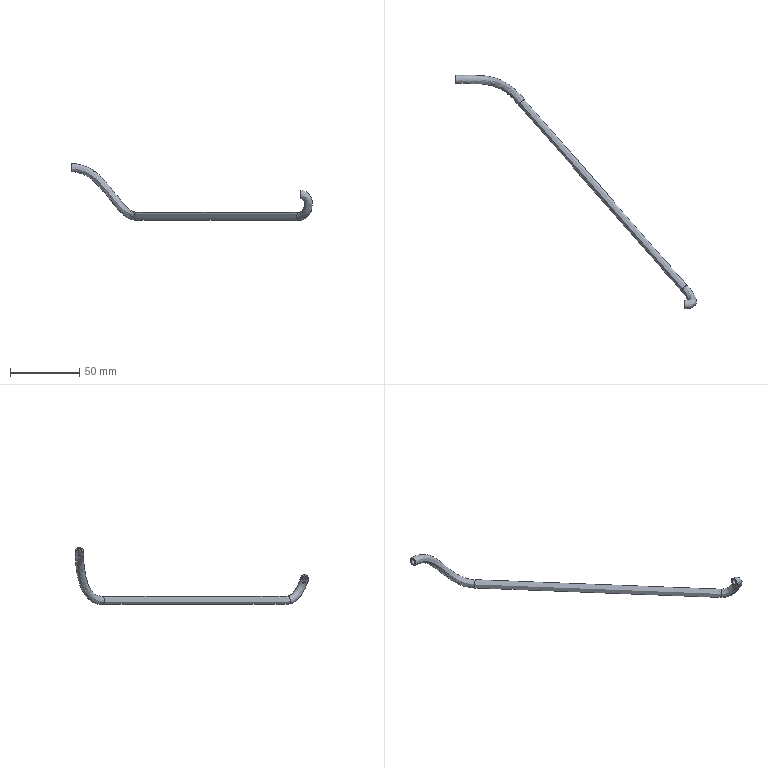Part | NX | features solid 2 | 1 solid | 8 faces | box 173.418 x 168.016 x 41.01 mm | volume 4216 mm3 | spline 6 | plane 2